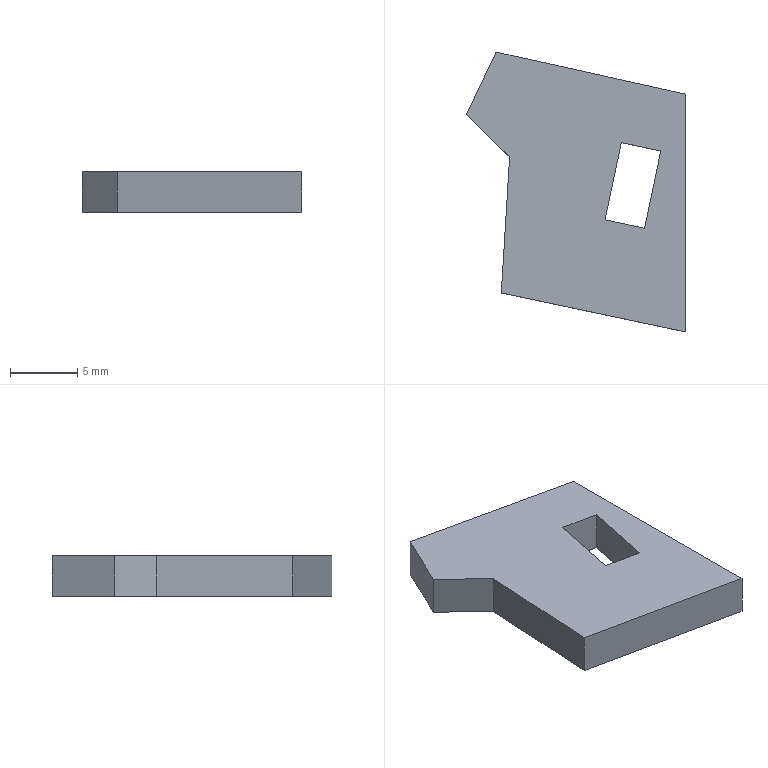Part | SolidWorks | features BaseBody 1 | 1 solid | 12 faces | box 16.323 x 20.843 x 3 mm | volume 699.822 mm3 | plane 7 | spline 5
STEP:
#1=CARTESIAN_POINT('',(16.74,-6.297,-1.5));
#2=VERTEX_POINT('',#1);
#3=CARTESIAN_POINT('',(17.958,-0.5428,-1.5));
#4=VERTEX_POINT('',#3);
#5=CARTESIAN_POINT('',(17.958,-0.5428,-1.5));
#6=DIRECTION('',(0.2071,0.9783,0.));
#7=VECTOR('',#6,1000.);
#8=LINE('',#5,#7);
#9=EDGE_CURVE('',#2,#4,#8,.T.);
#10=ORIENTED_EDGE('',*,*,#9,.F.);
#11=CARTESIAN_POINT('',(16.74,-6.297,1.5));
#12=VERTEX_POINT('',#11);
#13=CARTESIAN_POINT('',(16.74,-6.297,1.5));
#14=DIRECTION('',(0.,0.,-1.));
#15=VECTOR('',#14,1000.);
#16=LINE('',#13,#15);
#17=EDGE_CURVE('',#12,#2,#16,.T.);
#18=ORIENTED_EDGE('',*,*,#17,.F.);
#19=CARTESIAN_POINT('',(17.958,-0.5428,1.5));
#20=VERTEX_POINT('',#19);
#21=CARTESIAN_POINT('',(17.958,-0.5428,1.5));
#22=DIRECTION('',(0.2071,0.9783,0.));
#23=VECTOR('',#22,1000.);
#24=LINE('',#21,#23);
#25=EDGE_CURVE('',#12,#20,#24,.T.);
#26=ORIENTED_EDGE('',*,*,#25,.T.);
#27=CARTESIAN_POINT('',(17.958,-0.5428,1.5));
#28=DIRECTION('',(0.,0.,-1.));
#29=VECTOR('',#28,1000.);
#30=LINE('',#27,#29);
#31=EDGE_CURVE('',#20,#4,#30,.T.);
#32=ORIENTED_EDGE('',*,*,#31,.T.);
#33=EDGE_LOOP('',(#10,#18,#26,#32));
#34=FACE_OUTER_BOUND('',#33,.T.);
#35=CARTESIAN_POINT('',(17.958,-0.5428,1.5));
#36=DIRECTION('',(-0.9783,0.2071,0.));
#37=DIRECTION('',(0.,0.,1.));
#38=AXIS2_PLACEMENT_3D('',#35,#36,#37);
#39=PLANE('',#38);
#40=ADVANCED_FACE('',(#34),#39,.T.);
#41=CARTESIAN_POINT('',(13.805,-5.676,-1.5));
#42=VERTEX_POINT('',#41);
#43=CARTESIAN_POINT('',(16.74,-6.297,-1.5));
#44=DIRECTION('',(0.9783,-0.2071,0.));
#45=VECTOR('',#44,1000.);
#46=LINE('',#43,#45);
#47=EDGE_CURVE('',#42,#2,#46,.T.);
#48=ORIENTED_EDGE('',*,*,#47,.F.);
#49=CARTESIAN_POINT('',(13.805,-5.676,1.5));
#50=VERTEX_POINT('',#49);
#51=CARTESIAN_POINT('',(13.805,-5.676,1.5));
#52=DIRECTION('',(0.,0.,-1.));
#53=VECTOR('',#52,1000.);
#54=LINE('',#51,#53);
#55=EDGE_CURVE('',#50,#42,#54,.T.);
#56=ORIENTED_EDGE('',*,*,#55,.F.);
#57=CARTESIAN_POINT('',(16.74,-6.297,1.5));
#58=DIRECTION('',(0.9783,-0.2071,0.));
#59=VECTOR('',#58,1000.);
#60=LINE('',#57,#59);
#61=EDGE_CURVE('',#50,#12,#60,.T.);
#62=ORIENTED_EDGE('',*,*,#61,.T.);
#63=ORIENTED_EDGE('',*,*,#17,.T.);
#64=EDGE_LOOP('',(#48,#56,#62,#63));
#65=FACE_OUTER_BOUND('',#64,.T.);
#66=CARTESIAN_POINT('',(16.74,-6.297,1.5));
#67=DIRECTION('',(0.2071,0.9783,0.));
#68=DIRECTION('',(0.,0.,-1.));
#69=AXIS2_PLACEMENT_3D('',#66,#67,#68);
#70=PLANE('',#69);
#71=ADVANCED_FACE('',(#65),#70,.T.);
#72=CARTESIAN_POINT('',(15.023,0.07866,-1.5));
#73=VERTEX_POINT('',#72);
#74=CARTESIAN_POINT('',(15.023,0.07866,-1.5));
#75=DIRECTION('',(-0.2071,-0.9783,0.));
#76=VECTOR('',#75,1000.);
#77=LINE('',#74,#76);
#78=EDGE_CURVE('',#73,#42,#77,.T.);
#79=ORIENTED_EDGE('',*,*,#78,.F.);
#80=CARTESIAN_POINT('',(15.023,0.07866,1.5));
#81=VERTEX_POINT('',#80);
#82=CARTESIAN_POINT('',(15.023,0.07866,1.5));
#83=DIRECTION('',(0.,0.,-1.));
#84=VECTOR('',#83,1000.);
#85=LINE('',#82,#84);
#86=EDGE_CURVE('',#81,#73,#85,.T.);
#87=ORIENTED_EDGE('',*,*,#86,.F.);
#88=CARTESIAN_POINT('',(15.023,0.07866,1.5));
#89=DIRECTION('',(-0.2071,-0.9783,0.));
#90=VECTOR('',#89,1000.);
#91=LINE('',#88,#90);
#92=EDGE_CURVE('',#81,#50,#91,.T.);
#93=ORIENTED_EDGE('',*,*,#92,.T.);
#94=ORIENTED_EDGE('',*,*,#55,.T.);
#95=EDGE_LOOP('',(#79,#87,#93,#94));
#96=FACE_OUTER_BOUND('',#95,.T.);
#97=CARTESIAN_POINT('',(15.023,0.07866,1.5));
#98=DIRECTION('',(0.9783,-0.2071,0.));
#99=DIRECTION('',(0.,0.,-1.));
#100=AXIS2_PLACEMENT_3D('',#97,#98,#99);
#101=PLANE('',#100);
#102=ADVANCED_FACE('',(#96),#101,.T.);
#103=CARTESIAN_POINT('',(15.023,0.07866,-1.5));
#104=DIRECTION('',(-0.9783,0.2071,0.));
#105=VECTOR('',#104,1000.);
#106=LINE('',#103,#105);
#107=EDGE_CURVE('',#4,#73,#106,.T.);
#108=ORIENTED_EDGE('',*,*,#107,.F.);
#109=ORIENTED_EDGE('',*,*,#31,.F.);
#110=CARTESIAN_POINT('',(15.023,0.07866,1.5));
#111=DIRECTION('',(-0.9783,0.2071,0.));
#112=VECTOR('',#111,1000.);
#113=LINE('',#110,#112);
#114=EDGE_CURVE('',#20,#81,#113,.T.);
#115=ORIENTED_EDGE('',*,*,#114,.T.);
#116=ORIENTED_EDGE('',*,*,#86,.T.);
#117=EDGE_LOOP('',(#108,#109,#115,#116));
#118=FACE_OUTER_BOUND('',#117,.T.);
#119=CARTESIAN_POINT('',(15.023,0.07866,1.5));
#120=DIRECTION('',(-0.2071,-0.9783,0.));
#121=DIRECTION('',(-0.9783,0.2071,0.));
#122=AXIS2_PLACEMENT_3D('',#119,#120,#121);
#123=PLANE('',#122);
#124=ADVANCED_FACE('',(#118),#123,.T.);
#125=CARTESIAN_POINT('',(19.804,-14.018,-1.5));
#126=VERTEX_POINT('',#125);
#127=CARTESIAN_POINT('',(19.804,3.686,-1.5));
#128=VERTEX_POINT('',#127);
#129=CARTESIAN_POINT('',(19.804,3.686,-1.5));
#130=DIRECTION('',(0.,1.,0.));
#131=VECTOR('',#130,1000.);
#132=LINE('',#129,#131);
#133=EDGE_CURVE('',#126,#128,#132,.T.);
#134=ORIENTED_EDGE('',*,*,#133,.T.);
#135=CARTESIAN_POINT('',(19.804,3.686,1.5));
#136=VERTEX_POINT('',#135);
#137=CARTESIAN_POINT('',(19.804,3.686,1.5));
#138=DIRECTION('',(0.,0.,-1.));
#139=VECTOR('',#138,1000.);
#140=LINE('',#137,#139);
#141=EDGE_CURVE('',#136,#128,#140,.T.);
#142=ORIENTED_EDGE('',*,*,#141,.F.);
#143=CARTESIAN_POINT('',(19.804,-14.018,1.5));
#144=VERTEX_POINT('',#143);
#145=CARTESIAN_POINT('',(19.804,3.686,1.5));
#146=DIRECTION('',(0.,1.,0.));
#147=VECTOR('',#146,1000.);
#148=LINE('',#145,#147);
#149=EDGE_CURVE('',#144,#136,#148,.T.);
#150=ORIENTED_EDGE('',*,*,#149,.F.);
#151=CARTESIAN_POINT('',(19.804,-14.018,1.5));
#152=DIRECTION('',(0.,0.,-1.));
#153=VECTOR('',#152,1000.);
#154=LINE('',#151,#153);
#155=EDGE_CURVE('',#144,#126,#154,.T.);
#156=ORIENTED_EDGE('',*,*,#155,.T.);
#157=EDGE_LOOP('',(#134,#142,#150,#156));
#158=FACE_OUTER_BOUND('',#157,.T.);
#159=CARTESIAN_POINT('',(19.804,3.686,1.5));
#160=DIRECTION('',(-1.,0.,0.));
#161=DIRECTION('',(0.,0.,1.));
#162=AXIS2_PLACEMENT_3D('',#159,#160,#161);
#163=PLANE('',#162);
#164=ADVANCED_FACE('',(#158),#163,.F.);
#165=CARTESIAN_POINT('',(6.08,-11.115,-1.5));
#166=VERTEX_POINT('',#165);
#167=CARTESIAN_POINT('',(6.08,-11.115,-1.5));
#168=CARTESIAN_POINT('',(10.654,-12.083,-1.5));
#169=CARTESIAN_POINT('',(15.23,-13.051,-1.5));
#170=CARTESIAN_POINT('',(19.804,-14.018,-1.5));
#171=B_SPLINE_CURVE_WITH_KNOTS('',3,(#167,#168,#169,#170),.UNSPECIFIED.,.F.,.F.,(4,4),(0.7273,0.8182),.UNSPECIFIED.);
#172=EDGE_CURVE('',#166,#126,#171,.T.);
#173=ORIENTED_EDGE('',*,*,#172,.T.);
#174=ORIENTED_EDGE('',*,*,#155,.F.);
#175=CARTESIAN_POINT('',(6.08,-11.115,1.5));
#176=VERTEX_POINT('',#175);
#177=CARTESIAN_POINT('',(6.08,-11.115,1.5));
#178=CARTESIAN_POINT('',(10.654,-12.083,1.5));
#179=CARTESIAN_POINT('',(15.23,-13.051,1.5));
#180=CARTESIAN_POINT('',(19.804,-14.018,1.5));
#181=B_SPLINE_CURVE_WITH_KNOTS('',3,(#177,#178,#179,#180),.UNSPECIFIED.,.F.,.F.,(4,4),(0.7273,0.8182),.UNSPECIFIED.);
#182=EDGE_CURVE('',#176,#144,#181,.T.);
#183=ORIENTED_EDGE('',*,*,#182,.F.);
#184=CARTESIAN_POINT('',(6.08,-11.115,1.5));
#185=DIRECTION('',(0.,0.,-1.));
#186=VECTOR('',#185,1000.);
#187=LINE('',#184,#186);
#188=EDGE_CURVE('',#176,#166,#187,.T.);
#189=ORIENTED_EDGE('',*,*,#188,.T.);
#190=EDGE_LOOP('',(#173,#174,#183,#189));
#191=FACE_OUTER_BOUND('',#190,.T.);
#192=CARTESIAN_POINT('',(6.08,-11.115,1.5));
#193=CARTESIAN_POINT('',(6.08,-11.115,-1.5));
#194=CARTESIAN_POINT('',(10.654,-12.083,1.5));
#195=CARTESIAN_POINT('',(10.654,-12.083,-1.5));
#196=CARTESIAN_POINT('',(15.23,-13.051,1.5));
#197=CARTESIAN_POINT('',(15.23,-13.051,-1.5));
#198=CARTESIAN_POINT('',(19.804,-14.018,1.5));
#199=CARTESIAN_POINT('',(19.804,-14.018,-1.5));
#200=B_SPLINE_SURFACE_WITH_KNOTS('',3,1,((#192,#193),(#194,#195),(#196,#197),(#198,#199)),.UNSPECIFIED.,.F.,.F.,.F.,(4,4),(2,2),(0.7273,0.8182),(0.,1.),.UNSPECIFIED.);
#201=ADVANCED_FACE('',(#191),#200,.F.);
#202=CARTESIAN_POINT('',(6.7,-0.9851,-1.5));
#203=VERTEX_POINT('',#202);
#204=CARTESIAN_POINT('',(6.7,-0.9851,-1.5));
#205=CARTESIAN_POINT('',(6.494,-4.362,-1.5));
#206=CARTESIAN_POINT('',(6.286,-7.738,-1.5));
#207=CARTESIAN_POINT('',(6.08,-11.115,-1.5));
#208=B_SPLINE_CURVE_WITH_KNOTS('',3,(#204,#205,#206,#207),.UNSPECIFIED.,.F.,.F.,(4,4),(0.6364,0.7273),.UNSPECIFIED.);
#209=EDGE_CURVE('',#203,#166,#208,.T.);
#210=ORIENTED_EDGE('',*,*,#209,.T.);
#211=ORIENTED_EDGE('',*,*,#188,.F.);
#212=CARTESIAN_POINT('',(6.7,-0.9851,1.5));
#213=VERTEX_POINT('',#212);
#214=CARTESIAN_POINT('',(6.7,-0.9851,1.5));
#215=CARTESIAN_POINT('',(6.494,-4.362,1.5));
#216=CARTESIAN_POINT('',(6.286,-7.738,1.5));
#217=CARTESIAN_POINT('',(6.08,-11.115,1.5));
#218=B_SPLINE_CURVE_WITH_KNOTS('',3,(#214,#215,#216,#217),.UNSPECIFIED.,.F.,.F.,(4,4),(0.6364,0.7273),.UNSPECIFIED.);
#219=EDGE_CURVE('',#213,#176,#218,.T.);
#220=ORIENTED_EDGE('',*,*,#219,.F.);
#221=CARTESIAN_POINT('',(6.7,-0.9851,1.5));
#222=DIRECTION('',(0.,0.,-1.));
#223=VECTOR('',#222,1000.);
#224=LINE('',#221,#223);
#225=EDGE_CURVE('',#213,#203,#224,.T.);
#226=ORIENTED_EDGE('',*,*,#225,.T.);
#227=EDGE_LOOP('',(#210,#211,#220,#226));
#228=FACE_OUTER_BOUND('',#227,.T.);
#229=CARTESIAN_POINT('',(6.7,-0.9851,1.5));
#230=CARTESIAN_POINT('',(6.7,-0.9851,-1.5));
#231=CARTESIAN_POINT('',(6.494,-4.362,1.5));
#232=CARTESIAN_POINT('',(6.494,-4.362,-1.5));
#233=CARTESIAN_POINT('',(6.286,-7.738,1.5));
#234=CARTESIAN_POINT('',(6.286,-7.738,-1.5));
#235=CARTESIAN_POINT('',(6.08,-11.115,1.5));
#236=CARTESIAN_POINT('',(6.08,-11.115,-1.5));
#237=B_SPLINE_SURFACE_WITH_KNOTS('',3,1,((#229,#230),(#231,#232),(#233,#234),(#235,#236)),.UNSPECIFIED.,.F.,.F.,.F.,(4,4),(2,2),(0.6364,0.7273),(0.,1.),.UNSPECIFIED.);
#238=ADVANCED_FACE('',(#228),#237,.F.);
#239=CARTESIAN_POINT('',(3.481,2.16,-1.5));
#240=VERTEX_POINT('',#239);
#241=CARTESIAN_POINT('',(3.481,2.16,-1.5));
#242=CARTESIAN_POINT('',(4.555,1.111,-1.5));
#243=CARTESIAN_POINT('',(5.628,0.06296,-1.5));
#244=CARTESIAN_POINT('',(6.7,-0.9851,-1.5));
#245=B_SPLINE_CURVE_WITH_KNOTS('',3,(#241,#242,#243,#244),.UNSPECIFIED.,.F.,.F.,(4,4),(0.5455,0.6364),.UNSPECIFIED.);
#246=EDGE_CURVE('',#240,#203,#245,.T.);
#247=ORIENTED_EDGE('',*,*,#246,.T.);
#248=ORIENTED_EDGE('',*,*,#225,.F.);
#249=CARTESIAN_POINT('',(3.481,2.16,1.5));
#250=VERTEX_POINT('',#249);
#251=CARTESIAN_POINT('',(3.481,2.16,1.5));
#252=CARTESIAN_POINT('',(4.555,1.111,1.5));
#253=CARTESIAN_POINT('',(5.628,0.06296,1.5));
#254=CARTESIAN_POINT('',(6.7,-0.9851,1.5));
#255=B_SPLINE_CURVE_WITH_KNOTS('',3,(#251,#252,#253,#254),.UNSPECIFIED.,.F.,.F.,(4,4),(0.5455,0.6364),.UNSPECIFIED.);
#256=EDGE_CURVE('',#250,#213,#255,.T.);
#257=ORIENTED_EDGE('',*,*,#256,.F.);
#258=CARTESIAN_POINT('',(3.481,2.16,1.5));
#259=DIRECTION('',(0.,0.,-1.));
#260=VECTOR('',#259,1000.);
#261=LINE('',#258,#260);
#262=EDGE_CURVE('',#250,#240,#261,.T.);
#263=ORIENTED_EDGE('',*,*,#262,.T.);
#264=EDGE_LOOP('',(#247,#248,#257,#263));
#265=FACE_OUTER_BOUND('',#264,.T.);
#266=CARTESIAN_POINT('',(3.481,2.16,1.5));
#267=CARTESIAN_POINT('',(3.481,2.16,-1.5));
#268=CARTESIAN_POINT('',(4.555,1.111,1.5));
#269=CARTESIAN_POINT('',(4.555,1.111,-1.5));
#270=CARTESIAN_POINT('',(5.628,0.06296,1.5));
#271=CARTESIAN_POINT('',(5.628,0.06296,-1.5));
#272=CARTESIAN_POINT('',(6.7,-0.9851,1.5));
#273=CARTESIAN_POINT('',(6.7,-0.9851,-1.5));
#274=B_SPLINE_SURFACE_WITH_KNOTS('',3,1,((#266,#267),(#268,#269),(#270,#271),(#272,#273)),.UNSPECIFIED.,.F.,.F.,.F.,(4,4),(2,2),(0.5455,0.6364),(0.,1.),.UNSPECIFIED.);
#275=ADVANCED_FACE('',(#265),#274,.F.);
#276=CARTESIAN_POINT('',(5.681,6.825,-1.5));
#277=VERTEX_POINT('',#276);
#278=CARTESIAN_POINT('',(5.681,6.825,-1.5));
#279=CARTESIAN_POINT('',(4.945,5.269,-1.5));
#280=CARTESIAN_POINT('',(4.216,3.715,-1.5));
#281=CARTESIAN_POINT('',(3.481,2.16,-1.5));
#282=B_SPLINE_CURVE_WITH_KNOTS('',3,(#278,#279,#280,#281),.UNSPECIFIED.,.F.,.F.,(4,4),(0.4545,0.5455),.UNSPECIFIED.);
#283=EDGE_CURVE('',#277,#240,#282,.T.);
#284=ORIENTED_EDGE('',*,*,#283,.T.);
#285=ORIENTED_EDGE('',*,*,#262,.F.);
#286=CARTESIAN_POINT('',(5.681,6.825,1.5));
#287=VERTEX_POINT('',#286);
#288=CARTESIAN_POINT('',(5.681,6.825,1.5));
#289=CARTESIAN_POINT('',(4.945,5.269,1.5));
#290=CARTESIAN_POINT('',(4.216,3.715,1.5));
#291=CARTESIAN_POINT('',(3.481,2.16,1.5));
#292=B_SPLINE_CURVE_WITH_KNOTS('',3,(#288,#289,#290,#291),.UNSPECIFIED.,.F.,.F.,(4,4),(0.4545,0.5455),.UNSPECIFIED.);
#293=EDGE_CURVE('',#287,#250,#292,.T.);
#294=ORIENTED_EDGE('',*,*,#293,.F.);
#295=CARTESIAN_POINT('',(5.681,6.825,1.5));
#296=DIRECTION('',(0.,0.,-1.));
#297=VECTOR('',#296,1000.);
#298=LINE('',#295,#297);
#299=EDGE_CURVE('',#287,#277,#298,.T.);
#300=ORIENTED_EDGE('',*,*,#299,.T.);
#301=EDGE_LOOP('',(#284,#285,#294,#300));
#302=FACE_OUTER_BOUND('',#301,.T.);
#303=CARTESIAN_POINT('',(5.681,6.825,1.5));
#304=CARTESIAN_POINT('',(5.681,6.825,-1.5));
#305=CARTESIAN_POINT('',(4.945,5.269,1.5));
#306=CARTESIAN_POINT('',(4.945,5.269,-1.5));
#307=CARTESIAN_POINT('',(4.216,3.715,1.5));
#308=CARTESIAN_POINT('',(4.216,3.715,-1.5));
#309=CARTESIAN_POINT('',(3.481,2.16,1.5));
#310=CARTESIAN_POINT('',(3.481,2.16,-1.5));
#311=B_SPLINE_SURFACE_WITH_KNOTS('',3,1,((#303,#304),(#305,#306),(#307,#308),(#309,#310)),.UNSPECIFIED.,.F.,.F.,.F.,(4,4),(2,2),(0.4545,0.5455),(0.,1.),.UNSPECIFIED.);
#312=ADVANCED_FACE('',(#302),#311,.F.);
#313=CARTESIAN_POINT('',(19.804,3.686,-1.5));
#314=CARTESIAN_POINT('',(15.095,4.732,-1.5));
#315=CARTESIAN_POINT('',(10.389,5.779,-1.5));
#316=CARTESIAN_POINT('',(5.681,6.825,-1.5));
#317=B_SPLINE_CURVE_WITH_KNOTS('',3,(#313,#314,#315,#316),.UNSPECIFIED.,.F.,.F.,(4,4),(0.3636,0.4545),.UNSPECIFIED.);
#318=EDGE_CURVE('',#128,#277,#317,.T.);
#319=ORIENTED_EDGE('',*,*,#318,.T.);
#320=ORIENTED_EDGE('',*,*,#299,.F.);
#321=CARTESIAN_POINT('',(19.804,3.686,1.5));
#322=CARTESIAN_POINT('',(15.095,4.732,1.5));
#323=CARTESIAN_POINT('',(10.389,5.779,1.5));
#324=CARTESIAN_POINT('',(5.681,6.825,1.5));
#325=B_SPLINE_CURVE_WITH_KNOTS('',3,(#321,#322,#323,#324),.UNSPECIFIED.,.F.,.F.,(4,4),(0.3636,0.4545),.UNSPECIFIED.);
#326=EDGE_CURVE('',#136,#287,#325,.T.);
#327=ORIENTED_EDGE('',*,*,#326,.F.);
#328=ORIENTED_EDGE('',*,*,#141,.T.);
#329=EDGE_LOOP('',(#319,#320,#327,#328));
#330=FACE_OUTER_BOUND('',#329,.T.);
#331=CARTESIAN_POINT('',(19.804,3.686,1.5));
#332=CARTESIAN_POINT('',(19.804,3.686,-1.5));
#333=CARTESIAN_POINT('',(15.095,4.732,1.5));
#334=CARTESIAN_POINT('',(15.095,4.732,-1.5));
#335=CARTESIAN_POINT('',(10.389,5.779,1.5));
#336=CARTESIAN_POINT('',(10.389,5.779,-1.5));
#337=CARTESIAN_POINT('',(5.681,6.825,1.5));
#338=CARTESIAN_POINT('',(5.681,6.825,-1.5));
#339=B_SPLINE_SURFACE_WITH_KNOTS('',3,1,((#331,#332),(#333,#334),(#335,#336),(#337,#338)),.UNSPECIFIED.,.F.,.F.,.F.,(4,4),(2,2),(0.3636,0.4545),(0.,1.),.UNSPECIFIED.);
#340=ADVANCED_FACE('',(#330),#339,.F.);
#341=ORIENTED_EDGE('',*,*,#107,.T.);
#342=ORIENTED_EDGE('',*,*,#78,.T.);
#343=ORIENTED_EDGE('',*,*,#47,.T.);
#344=ORIENTED_EDGE('',*,*,#9,.T.);
#345=EDGE_LOOP('',(#341,#342,#343,#344));
#346=FACE_BOUND('',#345,.T.);
#347=ORIENTED_EDGE('',*,*,#318,.F.);
#348=ORIENTED_EDGE('',*,*,#133,.F.);
#349=ORIENTED_EDGE('',*,*,#172,.F.);
#350=ORIENTED_EDGE('',*,*,#209,.F.);
#351=ORIENTED_EDGE('',*,*,#246,.F.);
#352=ORIENTED_EDGE('',*,*,#283,.F.);
#353=EDGE_LOOP('',(#347,#348,#349,#350,#351,#352));
#354=FACE_OUTER_BOUND('',#353,.T.);
#355=CARTESIAN_POINT('',(12.742,5.255,-1.5));
#356=DIRECTION('',(0.,0.,1.));
#357=DIRECTION('',(1.,0.,0.));
#358=AXIS2_PLACEMENT_3D('',#355,#356,#357);
#359=PLANE('',#358);
#360=ADVANCED_FACE('',(#346,#354),#359,.F.);
#361=ORIENTED_EDGE('',*,*,#92,.F.);
#362=ORIENTED_EDGE('',*,*,#114,.F.);
#363=ORIENTED_EDGE('',*,*,#25,.F.);
#364=ORIENTED_EDGE('',*,*,#61,.F.);
#365=EDGE_LOOP('',(#361,#362,#363,#364));
#366=FACE_BOUND('',#365,.T.);
#367=ORIENTED_EDGE('',*,*,#326,.T.);
#368=ORIENTED_EDGE('',*,*,#293,.T.);
#369=ORIENTED_EDGE('',*,*,#256,.T.);
#370=ORIENTED_EDGE('',*,*,#219,.T.);
#371=ORIENTED_EDGE('',*,*,#182,.T.);
#372=ORIENTED_EDGE('',*,*,#149,.T.);
#373=EDGE_LOOP('',(#367,#368,#369,#370,#371,#372));
#374=FACE_OUTER_BOUND('',#373,.T.);
#375=CARTESIAN_POINT('',(12.742,5.255,1.5));
#376=DIRECTION('',(0.,0.,1.));
#377=DIRECTION('',(1.,0.,0.));
#378=AXIS2_PLACEMENT_3D('',#375,#376,#377);
#379=PLANE('',#378);
#380=ADVANCED_FACE('',(#366,#374),#379,.T.);
#381=CLOSED_SHELL('',(#40,#71,#102,#124,#164,#201,#238,#275,#312,#340,#360,#380));
#382=MANIFOLD_SOLID_BREP('',#381);
#383=CARTESIAN_POINT('',(0.,0.,0.));
#384=DIRECTION('',(0.,0.,1.));
#385=DIRECTION('',(1.,0.,0.));
#386=AXIS2_PLACEMENT_3D('',#383,#384,#385);
#387=(LENGTH_UNIT()NAMED_UNIT(*)SI_UNIT(.MILLI.,.METRE.));
#388=UNCERTAINTY_MEASURE_WITH_UNIT(LENGTH_MEASURE(0.00001),#387,'','');
#389=(NAMED_UNIT(*)PLANE_ANGLE_UNIT()SI_UNIT($,.RADIAN.));
#390=(NAMED_UNIT(*)SI_UNIT($,.STERADIAN.)SOLID_ANGLE_UNIT());
#391=(GEOMETRIC_REPRESENTATION_CONTEXT(3)GLOBAL_UNCERTAINTY_ASSIGNED_CONTEXT((#388))GLOBAL_UNIT_ASSIGNED_CONTEXT((#387,#389,#390))REPRESENTATION_CONTEXT('',''));
#392=ADVANCED_BREP_SHAPE_REPRESENTATION('',(#382,#386),#391);